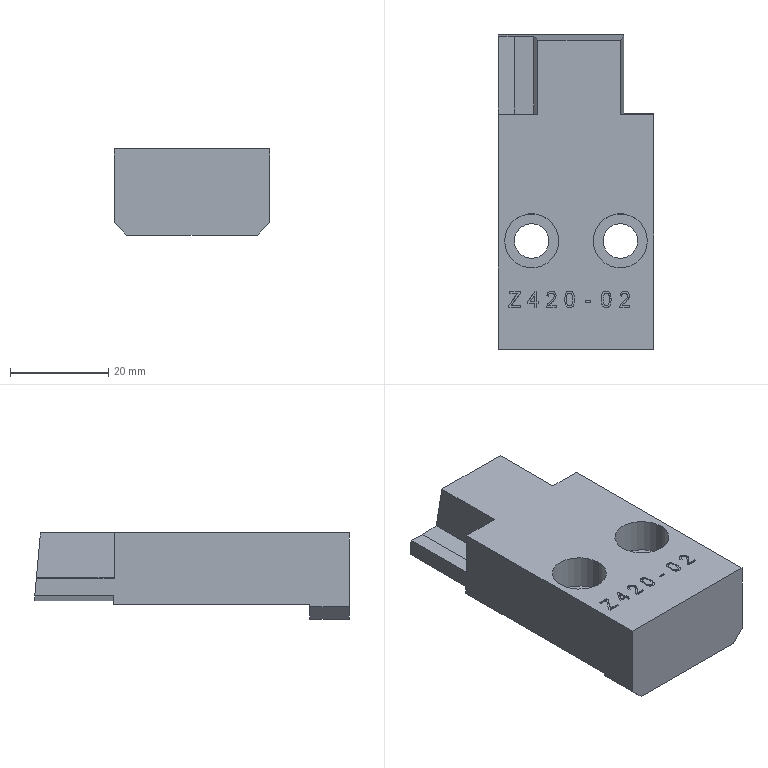Part | Creo | 1 solid | 151 faces | box 31.5 x 63.912 x 17.5 mm | volume 24713 mm3 | other 81 | plane 59 | cylinder 11 | commonest cylinder face diameters 7 x4 11 x4 2.89 x2 45.582 x1